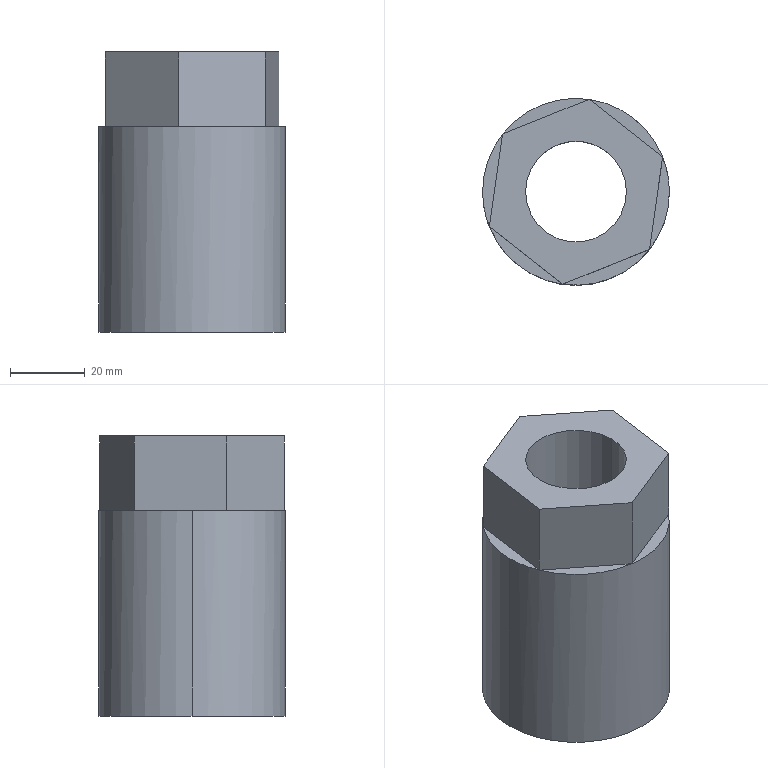Part | SolidWorks | features BaseBody 1 | 1 solid | 21 faces | box 50 x 50 x 75 mm | volume 76101 mm3 | plane 15 | cylinder 6 | commonest cylinder face diameters 27 x2 35 x2 50 x2
STEP:
#1=CARTESIAN_POINT('',(-92.145,49.565,55.));
#2=VERTEX_POINT('',#1);
#3=CARTESIAN_POINT('',(-90.343,40.243,55.));
#4=VERTEX_POINT('',#3);
#5=CARTESIAN_POINT('',(-115.343,40.243,55.));
#6=DIRECTION('',(0.,0.,-1.));
#7=DIRECTION('',(-1.,0.,0.));
#8=AXIS2_PLACEMENT_3D('',#5,#6,#7);
#9=CIRCLE('',#8,25.);
#10=EDGE_CURVE('',#2,#4,#9,.T.);
#11=ORIENTED_EDGE('',*,*,#10,.T.);
#12=CARTESIAN_POINT('',(-90.343,40.243,0.));
#13=VERTEX_POINT('',#12);
#14=CARTESIAN_POINT('',(-90.343,40.243,55.));
#15=DIRECTION('',(0.,0.,-1.));
#16=VECTOR('',#15,1000.);
#17=LINE('',#14,#16);
#18=EDGE_CURVE('',#4,#13,#17,.T.);
#19=ORIENTED_EDGE('',*,*,#18,.T.);
#20=CARTESIAN_POINT('',(-140.343,40.243,0.));
#21=VERTEX_POINT('',#20);
#22=CARTESIAN_POINT('',(-115.343,40.243,0.));
#23=DIRECTION('',(0.,0.,1.));
#24=DIRECTION('',(-1.,0.,0.));
#25=AXIS2_PLACEMENT_3D('',#22,#23,#24);
#26=CIRCLE('',#25,25.);
#27=EDGE_CURVE('',#13,#21,#26,.T.);
#28=ORIENTED_EDGE('',*,*,#27,.T.);
#29=CARTESIAN_POINT('',(-140.343,40.243,55.));
#30=VERTEX_POINT('',#29);
#31=CARTESIAN_POINT('',(-140.343,40.243,55.));
#32=DIRECTION('',(0.,0.,-1.));
#33=VECTOR('',#32,1000.);
#34=LINE('',#31,#33);
#35=EDGE_CURVE('',#30,#21,#34,.T.);
#36=ORIENTED_EDGE('',*,*,#35,.F.);
#37=CARTESIAN_POINT('',(-135.014,55.672,55.));
#38=VERTEX_POINT('',#37);
#39=CARTESIAN_POINT('',(-115.343,40.243,55.));
#40=DIRECTION('',(0.,0.,-1.));
#41=DIRECTION('',(-1.,0.,0.));
#42=AXIS2_PLACEMENT_3D('',#39,#40,#41);
#43=CIRCLE('',#42,25.);
#44=EDGE_CURVE('',#30,#38,#43,.T.);
#45=ORIENTED_EDGE('',*,*,#44,.T.);
#46=CARTESIAN_POINT('',(-111.817,64.993,55.));
#47=VERTEX_POINT('',#46);
#48=CARTESIAN_POINT('',(-115.343,40.243,55.));
#49=DIRECTION('',(0.,0.,-1.));
#50=DIRECTION('',(-1.,0.,0.));
#51=AXIS2_PLACEMENT_3D('',#48,#49,#50);
#52=CIRCLE('',#51,25.);
#53=EDGE_CURVE('',#38,#47,#52,.T.);
#54=ORIENTED_EDGE('',*,*,#53,.T.);
#55=CARTESIAN_POINT('',(-115.343,40.243,55.));
#56=DIRECTION('',(0.,0.,-1.));
#57=DIRECTION('',(-1.,0.,0.));
#58=AXIS2_PLACEMENT_3D('',#55,#56,#57);
#59=CIRCLE('',#58,25.);
#60=EDGE_CURVE('',#47,#2,#59,.T.);
#61=ORIENTED_EDGE('',*,*,#60,.T.);
#62=EDGE_LOOP('',(#11,#19,#28,#36,#45,#54,#61));
#63=FACE_OUTER_BOUND('',#62,.T.);
#64=CARTESIAN_POINT('',(-115.343,40.243,55.));
#65=DIRECTION('',(0.,0.,-1.));
#66=DIRECTION('',(-1.,0.,0.));
#67=AXIS2_PLACEMENT_3D('',#64,#65,#66);
#68=CYLINDRICAL_SURFACE('',#67,25.);
#69=ADVANCED_FACE('',(#63),#68,.T.);
#70=CARTESIAN_POINT('',(-97.843,40.243,55.));
#71=VERTEX_POINT('',#70);
#72=CARTESIAN_POINT('',(-132.843,40.243,55.));
#73=VERTEX_POINT('',#72);
#74=CARTESIAN_POINT('',(-115.343,40.243,55.));
#75=DIRECTION('',(0.,0.,-1.));
#76=DIRECTION('',(-1.,0.,0.));
#77=AXIS2_PLACEMENT_3D('',#74,#75,#76);
#78=CIRCLE('',#77,17.5);
#79=EDGE_CURVE('',#71,#73,#78,.T.);
#80=ORIENTED_EDGE('',*,*,#79,.F.);
#81=CARTESIAN_POINT('',(-97.843,40.243,0.));
#82=VERTEX_POINT('',#81);
#83=CARTESIAN_POINT('',(-97.843,40.243,55.));
#84=DIRECTION('',(0.,0.,-1.));
#85=VECTOR('',#84,1000.);
#86=LINE('',#83,#85);
#87=EDGE_CURVE('',#71,#82,#86,.T.);
#88=ORIENTED_EDGE('',*,*,#87,.T.);
#89=CARTESIAN_POINT('',(-132.843,40.243,0.));
#90=VERTEX_POINT('',#89);
#91=CARTESIAN_POINT('',(-115.343,40.243,0.));
#92=DIRECTION('',(0.,0.,-1.));
#93=DIRECTION('',(-1.,0.,0.));
#94=AXIS2_PLACEMENT_3D('',#91,#92,#93);
#95=CIRCLE('',#94,17.5);
#96=EDGE_CURVE('',#82,#90,#95,.T.);
#97=ORIENTED_EDGE('',*,*,#96,.T.);
#98=CARTESIAN_POINT('',(-132.843,40.243,55.));
#99=DIRECTION('',(0.,0.,-1.));
#100=VECTOR('',#99,1000.);
#101=LINE('',#98,#100);
#102=EDGE_CURVE('',#73,#90,#101,.T.);
#103=ORIENTED_EDGE('',*,*,#102,.F.);
#104=EDGE_LOOP('',(#80,#88,#97,#103));
#105=FACE_OUTER_BOUND('',#104,.T.);
#106=CARTESIAN_POINT('',(-115.343,40.243,55.));
#107=DIRECTION('',(0.,0.,-1.));
#108=DIRECTION('',(-1.,0.,0.));
#109=AXIS2_PLACEMENT_3D('',#106,#107,#108);
#110=CYLINDRICAL_SURFACE('',#109,17.5);
#111=ADVANCED_FACE('',(#105),#110,.F.);
#112=CARTESIAN_POINT('',(-101.843,40.243,75.));
#113=VERTEX_POINT('',#112);
#114=CARTESIAN_POINT('',(-128.843,40.243,75.));
#115=VERTEX_POINT('',#114);
#116=CARTESIAN_POINT('',(-115.343,40.243,75.));
#117=DIRECTION('',(0.,0.,-1.));
#118=DIRECTION('',(-1.,0.,0.));
#119=AXIS2_PLACEMENT_3D('',#116,#117,#118);
#120=CIRCLE('',#119,13.5);
#121=EDGE_CURVE('',#113,#115,#120,.T.);
#122=ORIENTED_EDGE('',*,*,#121,.F.);
#123=CARTESIAN_POINT('',(-101.843,40.243,55.));
#124=VERTEX_POINT('',#123);
#125=CARTESIAN_POINT('',(-101.843,40.243,75.));
#126=DIRECTION('',(0.,0.,-1.));
#127=VECTOR('',#126,1000.);
#128=LINE('',#125,#127);
#129=EDGE_CURVE('',#113,#124,#128,.T.);
#130=ORIENTED_EDGE('',*,*,#129,.T.);
#131=CARTESIAN_POINT('',(-128.843,40.243,55.));
#132=VERTEX_POINT('',#131);
#133=CARTESIAN_POINT('',(-115.343,40.243,55.));
#134=DIRECTION('',(0.,0.,-1.));
#135=DIRECTION('',(-1.,0.,0.));
#136=AXIS2_PLACEMENT_3D('',#133,#134,#135);
#137=CIRCLE('',#136,13.5);
#138=EDGE_CURVE('',#124,#132,#137,.T.);
#139=ORIENTED_EDGE('',*,*,#138,.T.);
#140=CARTESIAN_POINT('',(-128.843,40.243,75.));
#141=DIRECTION('',(0.,0.,-1.));
#142=VECTOR('',#141,1000.);
#143=LINE('',#140,#142);
#144=EDGE_CURVE('',#115,#132,#143,.T.);
#145=ORIENTED_EDGE('',*,*,#144,.F.);
#146=EDGE_LOOP('',(#122,#130,#139,#145));
#147=FACE_OUTER_BOUND('',#146,.T.);
#148=CARTESIAN_POINT('',(-115.343,40.243,75.));
#149=DIRECTION('',(0.,0.,-1.));
#150=DIRECTION('',(-1.,0.,0.));
#151=AXIS2_PLACEMENT_3D('',#148,#149,#150);
#152=CYLINDRICAL_SURFACE('',#151,13.5);
#153=ADVANCED_FACE('',(#147),#152,.F.);
#154=ORIENTED_EDGE('',*,*,#18,.F.);
#155=CARTESIAN_POINT('',(-95.671,24.815,55.));
#156=VERTEX_POINT('',#155);
#157=CARTESIAN_POINT('',(-115.343,40.243,55.));
#158=DIRECTION('',(0.,0.,-1.));
#159=DIRECTION('',(-1.,0.,0.));
#160=AXIS2_PLACEMENT_3D('',#157,#158,#159);
#161=CIRCLE('',#160,25.);
#162=EDGE_CURVE('',#4,#156,#161,.T.);
#163=ORIENTED_EDGE('',*,*,#162,.T.);
#164=CARTESIAN_POINT('',(-118.868,15.493,55.));
#165=VERTEX_POINT('',#164);
#166=CARTESIAN_POINT('',(-115.343,40.243,55.));
#167=DIRECTION('',(0.,0.,-1.));
#168=DIRECTION('',(-1.,0.,0.));
#169=AXIS2_PLACEMENT_3D('',#166,#167,#168);
#170=CIRCLE('',#169,25.);
#171=EDGE_CURVE('',#156,#165,#170,.T.);
#172=ORIENTED_EDGE('',*,*,#171,.T.);
#173=CARTESIAN_POINT('',(-138.54,30.921,55.));
#174=VERTEX_POINT('',#173);
#175=CARTESIAN_POINT('',(-115.343,40.243,55.));
#176=DIRECTION('',(0.,0.,-1.));
#177=DIRECTION('',(-1.,0.,0.));
#178=AXIS2_PLACEMENT_3D('',#175,#176,#177);
#179=CIRCLE('',#178,25.);
#180=EDGE_CURVE('',#165,#174,#179,.T.);
#181=ORIENTED_EDGE('',*,*,#180,.T.);
#182=CARTESIAN_POINT('',(-115.343,40.243,55.));
#183=DIRECTION('',(0.,0.,-1.));
#184=DIRECTION('',(-1.,0.,0.));
#185=AXIS2_PLACEMENT_3D('',#182,#183,#184);
#186=CIRCLE('',#185,25.);
#187=EDGE_CURVE('',#174,#30,#186,.T.);
#188=ORIENTED_EDGE('',*,*,#187,.T.);
#189=ORIENTED_EDGE('',*,*,#35,.T.);
#190=CARTESIAN_POINT('',(-115.343,40.243,0.));
#191=DIRECTION('',(0.,0.,1.));
#192=DIRECTION('',(-1.,0.,0.));
#193=AXIS2_PLACEMENT_3D('',#190,#191,#192);
#194=CIRCLE('',#193,25.);
#195=EDGE_CURVE('',#21,#13,#194,.T.);
#196=ORIENTED_EDGE('',*,*,#195,.T.);
#197=EDGE_LOOP('',(#154,#163,#172,#181,#188,#189,#196));
#198=FACE_OUTER_BOUND('',#197,.T.);
#199=CARTESIAN_POINT('',(-115.343,40.243,55.));
#200=DIRECTION('',(0.,0.,-1.));
#201=DIRECTION('',(-1.,0.,0.));
#202=AXIS2_PLACEMENT_3D('',#199,#200,#201);
#203=CYLINDRICAL_SURFACE('',#202,25.);
#204=ADVANCED_FACE('',(#198),#203,.T.);
#205=CARTESIAN_POINT('',(-111.817,64.993,55.));
#206=DIRECTION('',(0.7869,-0.6171,0.));
#207=VECTOR('',#206,1000.);
#208=LINE('',#205,#207);
#209=EDGE_CURVE('',#47,#2,#208,.T.);
#210=ORIENTED_EDGE('',*,*,#209,.T.);
#211=ORIENTED_EDGE('',*,*,#60,.F.);
#212=EDGE_LOOP('',(#210,#211));
#213=FACE_OUTER_BOUND('',#212,.T.);
#214=CARTESIAN_POINT('',(-115.343,40.243,55.));
#215=DIRECTION('',(0.,0.,1.));
#216=DIRECTION('',(1.,0.,0.));
#217=AXIS2_PLACEMENT_3D('',#214,#215,#216);
#218=PLANE('',#217);
#219=ADVANCED_FACE('',(#213),#218,.T.);
#220=CARTESIAN_POINT('',(-135.014,55.672,55.));
#221=DIRECTION('',(0.9279,0.3729,0.));
#222=VECTOR('',#221,1000.);
#223=LINE('',#220,#222);
#224=EDGE_CURVE('',#38,#47,#223,.T.);
#225=ORIENTED_EDGE('',*,*,#224,.T.);
#226=ORIENTED_EDGE('',*,*,#53,.F.);
#227=EDGE_LOOP('',(#225,#226));
#228=FACE_OUTER_BOUND('',#227,.T.);
#229=CARTESIAN_POINT('',(-115.343,40.243,55.));
#230=DIRECTION('',(0.,0.,1.));
#231=DIRECTION('',(1.,0.,0.));
#232=AXIS2_PLACEMENT_3D('',#229,#230,#231);
#233=PLANE('',#232);
#234=ADVANCED_FACE('',(#228),#233,.T.);
#235=ORIENTED_EDGE('',*,*,#187,.F.);
#236=CARTESIAN_POINT('',(-138.54,30.921,55.));
#237=DIRECTION('',(0.141,0.99,0.));
#238=VECTOR('',#237,1000.);
#239=LINE('',#236,#238);
#240=EDGE_CURVE('',#174,#38,#239,.T.);
#241=ORIENTED_EDGE('',*,*,#240,.T.);
#242=ORIENTED_EDGE('',*,*,#44,.F.);
#243=EDGE_LOOP('',(#235,#241,#242));
#244=FACE_OUTER_BOUND('',#243,.T.);
#245=CARTESIAN_POINT('',(-115.343,40.243,55.));
#246=DIRECTION('',(0.,0.,1.));
#247=DIRECTION('',(1.,0.,0.));
#248=AXIS2_PLACEMENT_3D('',#245,#246,#247);
#249=PLANE('',#248);
#250=ADVANCED_FACE('',(#244),#249,.T.);
#251=CARTESIAN_POINT('',(-115.343,40.243,0.));
#252=DIRECTION('',(0.,0.,-1.));
#253=DIRECTION('',(-1.,0.,0.));
#254=AXIS2_PLACEMENT_3D('',#251,#252,#253);
#255=CIRCLE('',#254,17.5);
#256=EDGE_CURVE('',#90,#82,#255,.T.);
#257=ORIENTED_EDGE('',*,*,#256,.F.);
#258=ORIENTED_EDGE('',*,*,#96,.F.);
#259=EDGE_LOOP('',(#257,#258));
#260=FACE_BOUND('',#259,.T.);
#261=ORIENTED_EDGE('',*,*,#195,.F.);
#262=ORIENTED_EDGE('',*,*,#27,.F.);
#263=EDGE_LOOP('',(#261,#262));
#264=FACE_OUTER_BOUND('',#263,.T.);
#265=CARTESIAN_POINT('',(-115.343,40.243,0.));
#266=DIRECTION('',(0.,0.,1.));
#267=DIRECTION('',(1.,0.,0.));
#268=AXIS2_PLACEMENT_3D('',#265,#266,#267);
#269=PLANE('',#268);
#270=ADVANCED_FACE('',(#260,#264),#269,.F.);
#271=CARTESIAN_POINT('',(-92.145,49.565,55.));
#272=DIRECTION('',(-0.141,-0.99,0.));
#273=VECTOR('',#272,1000.);
#274=LINE('',#271,#273);
#275=EDGE_CURVE('',#2,#156,#274,.T.);
#276=ORIENTED_EDGE('',*,*,#275,.T.);
#277=ORIENTED_EDGE('',*,*,#162,.F.);
#278=ORIENTED_EDGE('',*,*,#10,.F.);
#279=EDGE_LOOP('',(#276,#277,#278));
#280=FACE_OUTER_BOUND('',#279,.T.);
#281=CARTESIAN_POINT('',(-115.343,40.243,55.));
#282=DIRECTION('',(0.,0.,1.));
#283=DIRECTION('',(1.,0.,0.));
#284=AXIS2_PLACEMENT_3D('',#281,#282,#283);
#285=PLANE('',#284);
#286=ADVANCED_FACE('',(#280),#285,.T.);
#287=CARTESIAN_POINT('',(-111.817,64.993,75.));
#288=VERTEX_POINT('',#287);
#289=CARTESIAN_POINT('',(-111.817,64.993,75.));
#290=DIRECTION('',(0.,0.,-1.));
#291=VECTOR('',#290,1000.);
#292=LINE('',#289,#291);
#293=EDGE_CURVE('',#288,#47,#292,.T.);
#294=ORIENTED_EDGE('',*,*,#293,.F.);
#295=CARTESIAN_POINT('',(-92.145,49.565,75.));
#296=VERTEX_POINT('',#295);
#297=CARTESIAN_POINT('',(-92.145,49.565,75.));
#298=DIRECTION('',(-0.7869,0.6171,0.));
#299=VECTOR('',#298,1000.);
#300=LINE('',#297,#299);
#301=EDGE_CURVE('',#296,#288,#300,.T.);
#302=ORIENTED_EDGE('',*,*,#301,.F.);
#303=CARTESIAN_POINT('',(-92.145,49.565,75.));
#304=DIRECTION('',(0.,0.,1.));
#305=VECTOR('',#304,1000.);
#306=LINE('',#303,#305);
#307=EDGE_CURVE('',#2,#296,#306,.T.);
#308=ORIENTED_EDGE('',*,*,#307,.F.);
#309=ORIENTED_EDGE('',*,*,#209,.F.);
#310=EDGE_LOOP('',(#294,#302,#308,#309));
#311=FACE_OUTER_BOUND('',#310,.T.);
#312=CARTESIAN_POINT('',(-92.145,49.565,75.));
#313=DIRECTION('',(-0.6171,-0.7869,0.));
#314=DIRECTION('',(0.7869,-0.6171,0.));
#315=AXIS2_PLACEMENT_3D('',#312,#313,#314);
#316=PLANE('',#315);
#317=ADVANCED_FACE('',(#311),#316,.F.);
#318=CARTESIAN_POINT('',(-135.014,55.672,75.));
#319=VERTEX_POINT('',#318);
#320=CARTESIAN_POINT('',(-135.014,55.672,75.));
#321=DIRECTION('',(0.,0.,-1.));
#322=VECTOR('',#321,1000.);
#323=LINE('',#320,#322);
#324=EDGE_CURVE('',#319,#38,#323,.T.);
#325=ORIENTED_EDGE('',*,*,#324,.F.);
#326=CARTESIAN_POINT('',(-111.817,64.993,75.));
#327=DIRECTION('',(-0.9279,-0.3729,0.));
#328=VECTOR('',#327,1000.);
#329=LINE('',#326,#328);
#330=EDGE_CURVE('',#288,#319,#329,.T.);
#331=ORIENTED_EDGE('',*,*,#330,.F.);
#332=ORIENTED_EDGE('',*,*,#293,.T.);
#333=ORIENTED_EDGE('',*,*,#224,.F.);
#334=EDGE_LOOP('',(#325,#331,#332,#333));
#335=FACE_OUTER_BOUND('',#334,.T.);
#336=CARTESIAN_POINT('',(-111.817,64.993,75.));
#337=DIRECTION('',(0.3729,-0.9279,0.));
#338=DIRECTION('',(0.9279,0.3729,0.));
#339=AXIS2_PLACEMENT_3D('',#336,#337,#338);
#340=PLANE('',#339);
#341=ADVANCED_FACE('',(#335),#340,.F.);
#342=CARTESIAN_POINT('',(-138.54,30.921,75.));
#343=VERTEX_POINT('',#342);
#344=CARTESIAN_POINT('',(-138.54,30.921,75.));
#345=DIRECTION('',(0.,0.,-1.));
#346=VECTOR('',#345,1000.);
#347=LINE('',#344,#346);
#348=EDGE_CURVE('',#343,#174,#347,.T.);
#349=ORIENTED_EDGE('',*,*,#348,.F.);
#350=CARTESIAN_POINT('',(-135.014,55.672,75.));
#351=DIRECTION('',(-0.141,-0.99,0.));
#352=VECTOR('',#351,1000.);
#353=LINE('',#350,#352);
#354=EDGE_CURVE('',#319,#343,#353,.T.);
#355=ORIENTED_EDGE('',*,*,#354,.F.);
#356=ORIENTED_EDGE('',*,*,#324,.T.);
#357=ORIENTED_EDGE('',*,*,#240,.F.);
#358=EDGE_LOOP('',(#349,#355,#356,#357));
#359=FACE_OUTER_BOUND('',#358,.T.);
#360=CARTESIAN_POINT('',(-135.014,55.672,75.));
#361=DIRECTION('',(0.99,-0.141,0.));
#362=DIRECTION('',(0.141,0.99,0.));
#363=AXIS2_PLACEMENT_3D('',#360,#361,#362);
#364=PLANE('',#363);
#365=ADVANCED_FACE('',(#359),#364,.F.);
#366=CARTESIAN_POINT('',(-118.868,15.493,55.));
#367=DIRECTION('',(-0.7869,0.6171,0.));
#368=VECTOR('',#367,1000.);
#369=LINE('',#366,#368);
#370=EDGE_CURVE('',#165,#174,#369,.T.);
#371=ORIENTED_EDGE('',*,*,#370,.T.);
#372=ORIENTED_EDGE('',*,*,#180,.F.);
#373=EDGE_LOOP('',(#371,#372));
#374=FACE_OUTER_BOUND('',#373,.T.);
#375=CARTESIAN_POINT('',(-115.343,40.243,55.));
#376=DIRECTION('',(0.,0.,1.));
#377=DIRECTION('',(1.,0.,0.));
#378=AXIS2_PLACEMENT_3D('',#375,#376,#377);
#379=PLANE('',#378);
#380=ADVANCED_FACE('',(#374),#379,.T.);
#381=CARTESIAN_POINT('',(-95.671,24.815,55.));
#382=DIRECTION('',(-0.9279,-0.3729,0.));
#383=VECTOR('',#382,1000.);
#384=LINE('',#381,#383);
#385=EDGE_CURVE('',#156,#165,#384,.T.);
#386=ORIENTED_EDGE('',*,*,#385,.T.);
#387=ORIENTED_EDGE('',*,*,#171,.F.);
#388=EDGE_LOOP('',(#386,#387));
#389=FACE_OUTER_BOUND('',#388,.T.);
#390=CARTESIAN_POINT('',(-115.343,40.243,55.));
#391=DIRECTION('',(0.,0.,1.));
#392=DIRECTION('',(1.,0.,0.));
#393=AXIS2_PLACEMENT_3D('',#390,#391,#392);
#394=PLANE('',#393);
#395=ADVANCED_FACE('',(#389),#394,.T.);
#396=ORIENTED_EDGE('',*,*,#87,.F.);
#397=CARTESIAN_POINT('',(-115.343,40.243,55.));
#398=DIRECTION('',(0.,0.,-1.));
#399=DIRECTION('',(-1.,0.,0.));
#400=AXIS2_PLACEMENT_3D('',#397,#398,#399);
#401=CIRCLE('',#400,17.5);
#402=EDGE_CURVE('',#73,#71,#401,.T.);
#403=ORIENTED_EDGE('',*,*,#402,.F.);
#404=ORIENTED_EDGE('',*,*,#102,.T.);
#405=ORIENTED_EDGE('',*,*,#256,.T.);
#406=EDGE_LOOP('',(#396,#403,#404,#405));
#407=FACE_OUTER_BOUND('',#406,.T.);
#408=CARTESIAN_POINT('',(-115.343,40.243,55.));
#409=DIRECTION('',(0.,0.,-1.));
#410=DIRECTION('',(-1.,0.,0.));
#411=AXIS2_PLACEMENT_3D('',#408,#409,#410);
#412=CYLINDRICAL_SURFACE('',#411,17.5);
#413=ADVANCED_FACE('',(#407),#412,.F.);
#414=ORIENTED_EDGE('',*,*,#307,.T.);
#415=CARTESIAN_POINT('',(-95.671,24.815,75.));
#416=VERTEX_POINT('',#415);
#417=CARTESIAN_POINT('',(-95.671,24.815,75.));
#418=DIRECTION('',(0.141,0.99,0.));
#419=VECTOR('',#418,1000.);
#420=LINE('',#417,#419);
#421=EDGE_CURVE('',#416,#296,#420,.T.);
#422=ORIENTED_EDGE('',*,*,#421,.F.);
#423=CARTESIAN_POINT('',(-95.671,24.815,75.));
#424=DIRECTION('',(0.,0.,1.));
#425=VECTOR('',#424,1000.);
#426=LINE('',#423,#425);
#427=EDGE_CURVE('',#156,#416,#426,.T.);
#428=ORIENTED_EDGE('',*,*,#427,.F.);
#429=ORIENTED_EDGE('',*,*,#275,.F.);
#430=EDGE_LOOP('',(#414,#422,#428,#429));
#431=FACE_OUTER_BOUND('',#430,.T.);
#432=CARTESIAN_POINT('',(-95.671,24.815,75.));
#433=DIRECTION('',(-0.99,0.141,0.));
#434=DIRECTION('',(-0.141,-0.99,0.));
#435=AXIS2_PLACEMENT_3D('',#432,#433,#434);
#436=PLANE('',#435);
#437=ADVANCED_FACE('',(#431),#436,.F.);
#438=CARTESIAN_POINT('',(-115.343,40.243,75.));
#439=DIRECTION('',(0.,0.,-1.));
#440=DIRECTION('',(-1.,0.,0.));
#441=AXIS2_PLACEMENT_3D('',#438,#439,#440);
#442=CIRCLE('',#441,13.5);
#443=EDGE_CURVE('',#115,#113,#442,.T.);
#444=ORIENTED_EDGE('',*,*,#443,.T.);
#445=ORIENTED_EDGE('',*,*,#121,.T.);
#446=EDGE_LOOP('',(#444,#445));
#447=FACE_BOUND('',#446,.T.);
#448=ORIENTED_EDGE('',*,*,#301,.T.);
#449=ORIENTED_EDGE('',*,*,#330,.T.);
#450=ORIENTED_EDGE('',*,*,#354,.T.);
#451=CARTESIAN_POINT('',(-118.868,15.493,75.));
#452=VERTEX_POINT('',#451);
#453=CARTESIAN_POINT('',(-138.54,30.921,75.));
#454=DIRECTION('',(0.7869,-0.6171,0.));
#455=VECTOR('',#454,1000.);
#456=LINE('',#453,#455);
#457=EDGE_CURVE('',#343,#452,#456,.T.);
#458=ORIENTED_EDGE('',*,*,#457,.T.);
#459=CARTESIAN_POINT('',(-118.868,15.493,75.));
#460=DIRECTION('',(0.9279,0.3729,0.));
#461=VECTOR('',#460,1000.);
#462=LINE('',#459,#461);
#463=EDGE_CURVE('',#452,#416,#462,.T.);
#464=ORIENTED_EDGE('',*,*,#463,.T.);
#465=ORIENTED_EDGE('',*,*,#421,.T.);
#466=EDGE_LOOP('',(#448,#449,#450,#458,#464,#465));
#467=FACE_OUTER_BOUND('',#466,.T.);
#468=CARTESIAN_POINT('',(0.,0.,75.));
#469=DIRECTION('',(0.,0.,1.));
#470=DIRECTION('',(1.,0.,0.));
#471=AXIS2_PLACEMENT_3D('',#468,#469,#470);
#472=PLANE('',#471);
#473=ADVANCED_FACE('',(#447,#467),#472,.T.);
#474=CARTESIAN_POINT('',(-118.868,15.493,75.));
#475=DIRECTION('',(0.,0.,-1.));
#476=VECTOR('',#475,1000.);
#477=LINE('',#474,#476);
#478=EDGE_CURVE('',#452,#165,#477,.T.);
#479=ORIENTED_EDGE('',*,*,#478,.F.);
#480=ORIENTED_EDGE('',*,*,#457,.F.);
#481=ORIENTED_EDGE('',*,*,#348,.T.);
#482=ORIENTED_EDGE('',*,*,#370,.F.);
#483=EDGE_LOOP('',(#479,#480,#481,#482));
#484=FACE_OUTER_BOUND('',#483,.T.);
#485=CARTESIAN_POINT('',(-138.54,30.921,75.));
#486=DIRECTION('',(0.6171,0.7869,0.));
#487=DIRECTION('',(-0.7869,0.6171,0.));
#488=AXIS2_PLACEMENT_3D('',#485,#486,#487);
#489=PLANE('',#488);
#490=ADVANCED_FACE('',(#484),#489,.F.);
#491=ORIENTED_EDGE('',*,*,#427,.T.);
#492=ORIENTED_EDGE('',*,*,#463,.F.);
#493=ORIENTED_EDGE('',*,*,#478,.T.);
#494=ORIENTED_EDGE('',*,*,#385,.F.);
#495=EDGE_LOOP('',(#491,#492,#493,#494));
#496=FACE_OUTER_BOUND('',#495,.T.);
#497=CARTESIAN_POINT('',(-118.868,15.493,75.));
#498=DIRECTION('',(-0.3729,0.9279,0.));
#499=DIRECTION('',(-0.9279,-0.3729,0.));
#500=AXIS2_PLACEMENT_3D('',#497,#498,#499);
#501=PLANE('',#500);
#502=ADVANCED_FACE('',(#496),#501,.F.);
#503=CARTESIAN_POINT('',(-115.343,40.243,55.));
#504=DIRECTION('',(0.,0.,-1.));
#505=DIRECTION('',(-1.,0.,0.));
#506=AXIS2_PLACEMENT_3D('',#503,#504,#505);
#507=CIRCLE('',#506,13.5);
#508=EDGE_CURVE('',#132,#124,#507,.T.);
#509=ORIENTED_EDGE('',*,*,#508,.F.);
#510=ORIENTED_EDGE('',*,*,#138,.F.);
#511=EDGE_LOOP('',(#509,#510));
#512=FACE_BOUND('',#511,.T.);
#513=ORIENTED_EDGE('',*,*,#402,.T.);
#514=ORIENTED_EDGE('',*,*,#79,.T.);
#515=EDGE_LOOP('',(#513,#514));
#516=FACE_OUTER_BOUND('',#515,.T.);
#517=CARTESIAN_POINT('',(0.,0.,55.));
#518=DIRECTION('',(0.,0.,1.));
#519=DIRECTION('',(1.,0.,0.));
#520=AXIS2_PLACEMENT_3D('',#517,#518,#519);
#521=PLANE('',#520);
#522=ADVANCED_FACE('',(#512,#516),#521,.F.);
#523=ORIENTED_EDGE('',*,*,#129,.F.);
#524=ORIENTED_EDGE('',*,*,#443,.F.);
#525=ORIENTED_EDGE('',*,*,#144,.T.);
#526=ORIENTED_EDGE('',*,*,#508,.T.);
#527=EDGE_LOOP('',(#523,#524,#525,#526));
#528=FACE_OUTER_BOUND('',#527,.T.);
#529=CARTESIAN_POINT('',(-115.343,40.243,75.));
#530=DIRECTION('',(0.,0.,-1.));
#531=DIRECTION('',(-1.,0.,0.));
#532=AXIS2_PLACEMENT_3D('',#529,#530,#531);
#533=CYLINDRICAL_SURFACE('',#532,13.5);
#534=ADVANCED_FACE('',(#528),#533,.F.);
#535=CLOSED_SHELL('',(#69,#111,#153,#204,#219,#234,#250,#270,#286,#317,#341,#365,#380,#395,#413,#437,#473,#490,#502,#522,#534));
#536=MANIFOLD_SOLID_BREP('',#535);
#537=CARTESIAN_POINT('',(0.,0.,0.));
#538=DIRECTION('',(0.,0.,1.));
#539=DIRECTION('',(1.,0.,0.));
#540=AXIS2_PLACEMENT_3D('',#537,#538,#539);
#541=(LENGTH_UNIT()NAMED_UNIT(*)SI_UNIT(.MILLI.,.METRE.));
#542=UNCERTAINTY_MEASURE_WITH_UNIT(LENGTH_MEASURE(0.00001),#541,'','');
#543=(NAMED_UNIT(*)PLANE_ANGLE_UNIT()SI_UNIT($,.RADIAN.));
#544=(NAMED_UNIT(*)SI_UNIT($,.STERADIAN.)SOLID_ANGLE_UNIT());
#545=(GEOMETRIC_REPRESENTATION_CONTEXT(3)GLOBAL_UNCERTAINTY_ASSIGNED_CONTEXT((#542))GLOBAL_UNIT_ASSIGNED_CONTEXT((#541,#543,#544))REPRESENTATION_CONTEXT('',''));
#546=ADVANCED_BREP_SHAPE_REPRESENTATION('',(#536,#540),#545);